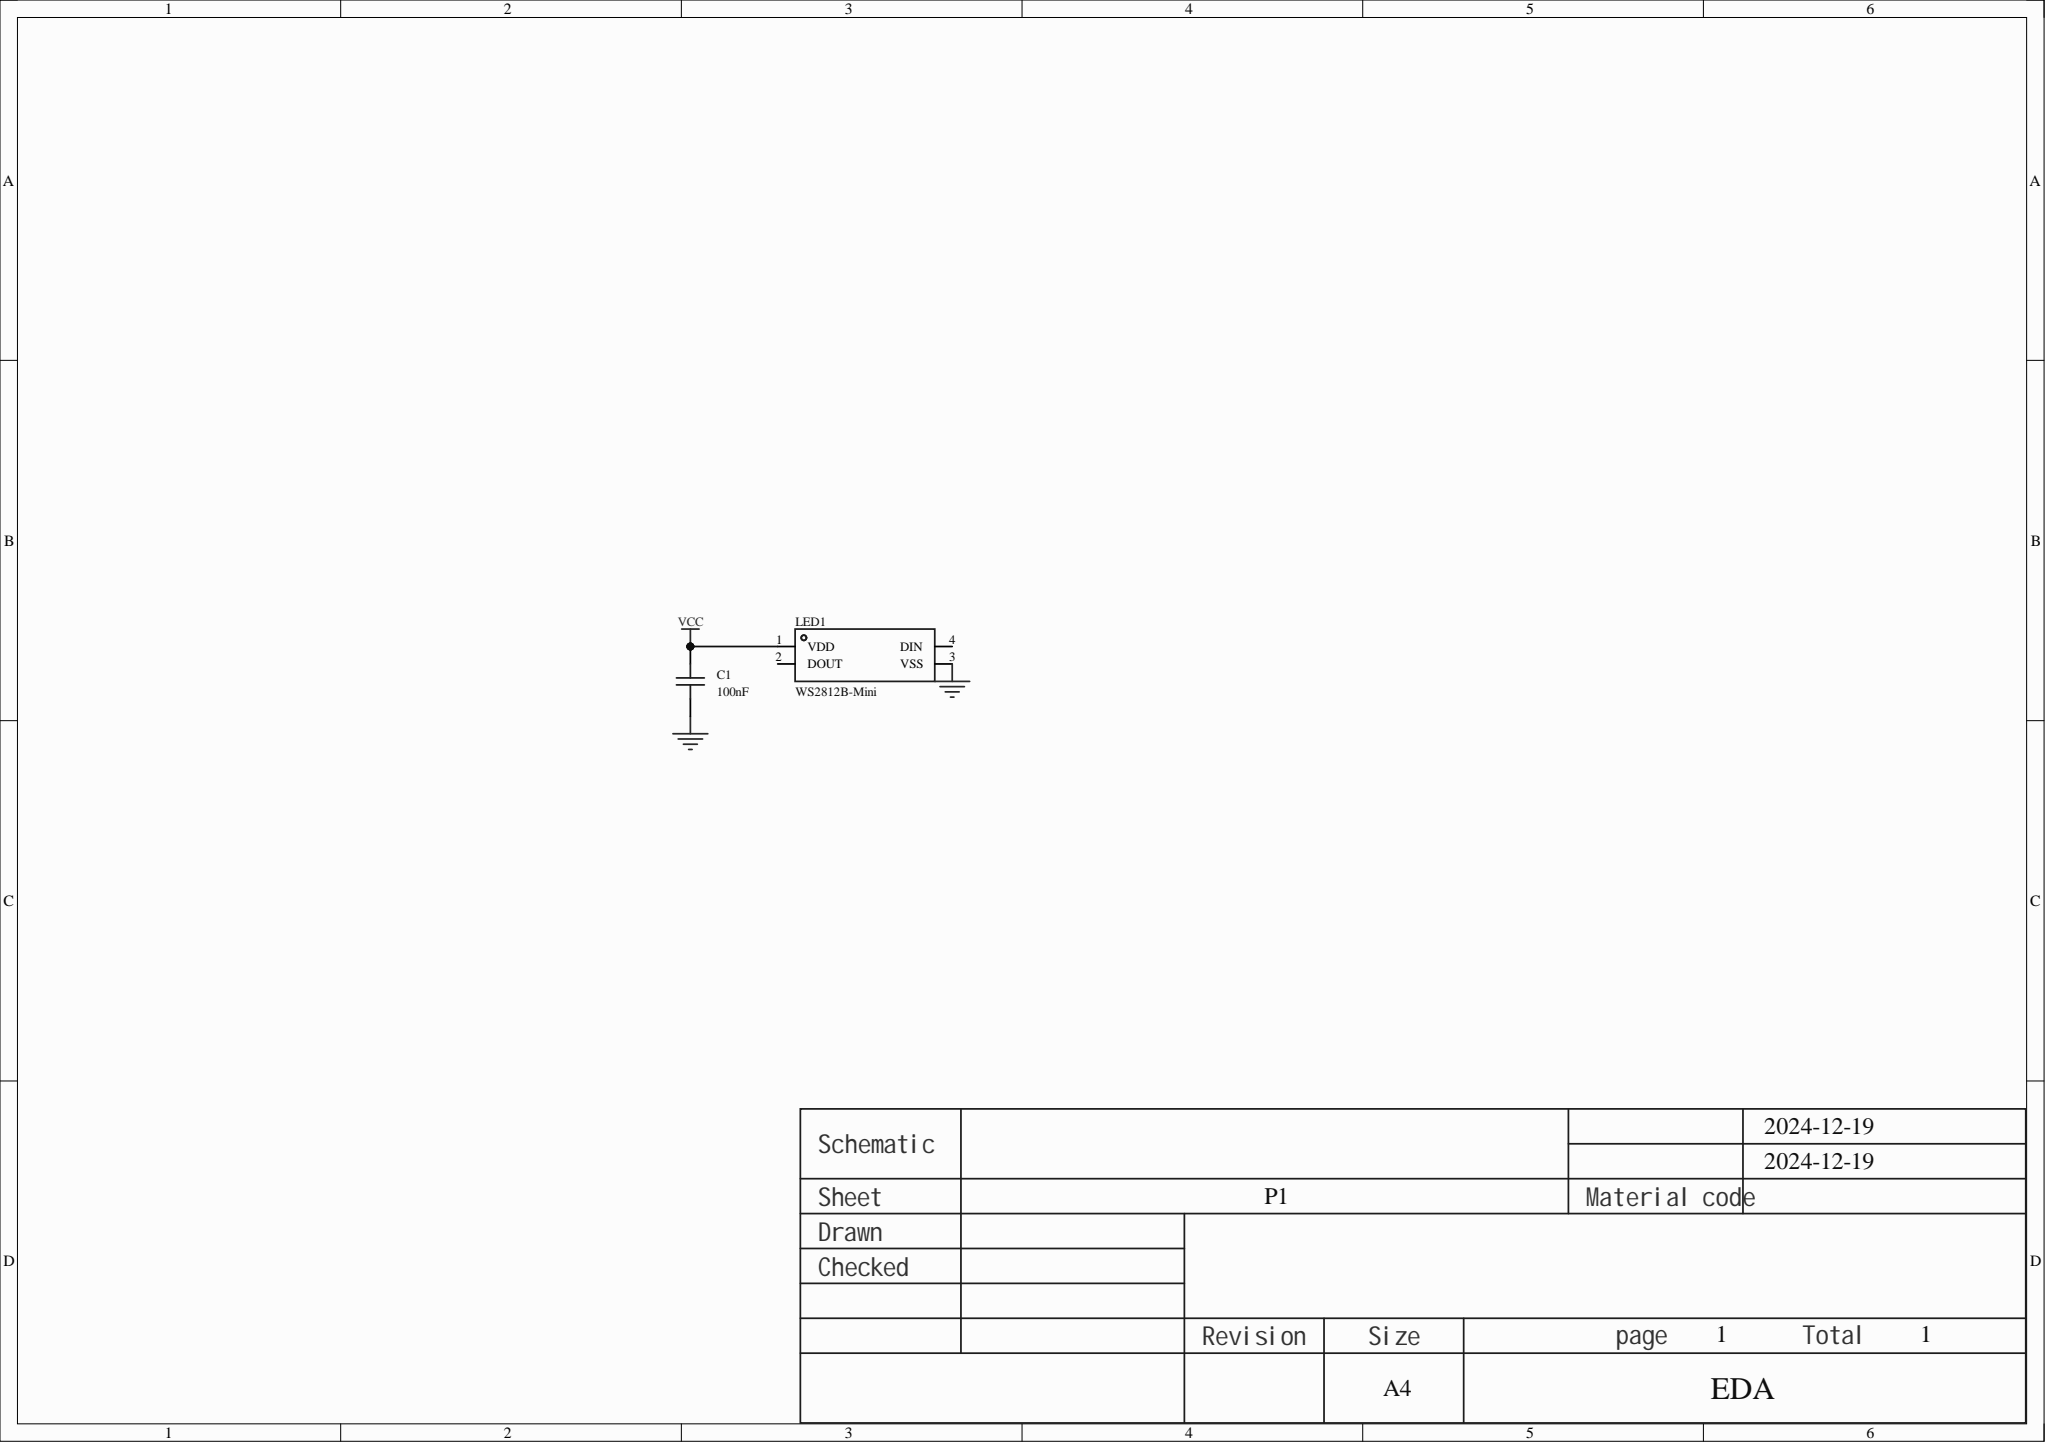Circuit board | Altium Designer | 2 parts | 2 nets
Bill of materials:
Comment,Description,Designator,Footprint,LibRef,Quantity
"100nF","","C1","C0603","CAP_0603","1"
"WS2812B-Mini","(moisture sensitive: see datasheet for details)","LED1","LED-SMD_4P-L3.5-W3.5-TL_WS2812B","WS2812B-Mini","1"
Netlist (Protel format):
[
C1
C0603
100nF



]
[
LED1
LED-SMD_4P-L3.5-W3.5-TL_WS2812B
WS2812B-Mini



]
(
VCC
C1-2
LED1-1
)
(
GND
C1-1
LED1-3
)